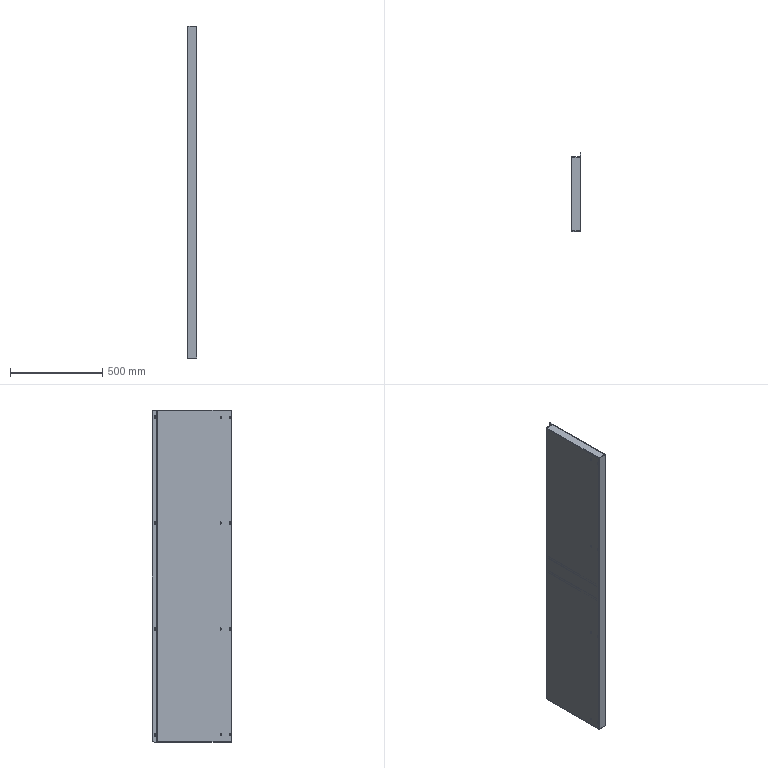Part | SolidWorks | 2 solids | 198 faces | box 50 x 430 x 1800 mm | volume 1681113 mm3 | plane 130 | cylinder 64 | spline 4 | commonest cylinder face diameters 6 x16 2 x13 5 x13 7 x12 8 x8 20 x2